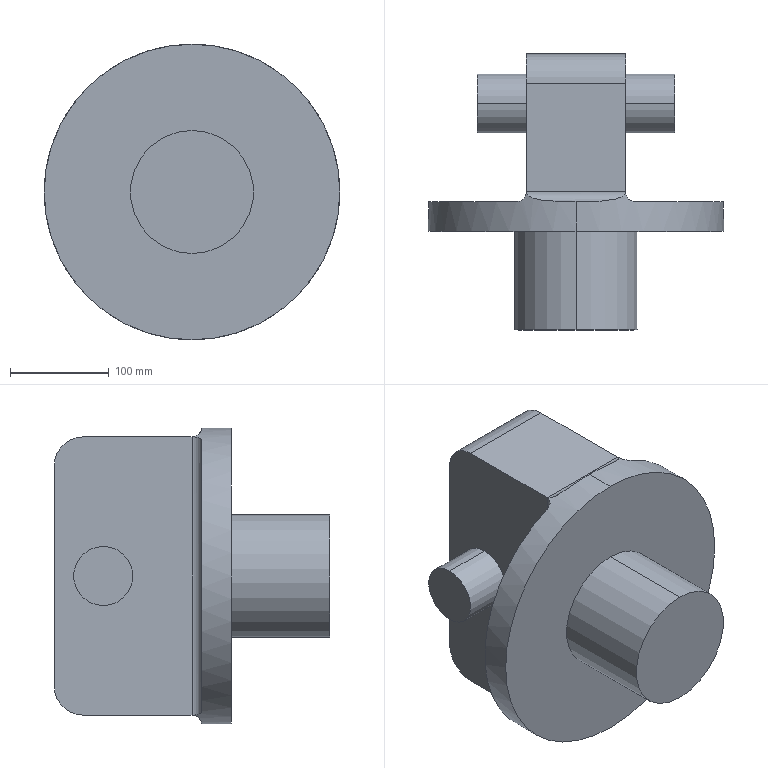Part | SolidWorks | features Revolution 3, ICE 2, BaseBody 1, Fillet 1 | 4 solids | 28 faces | box 300 x 280 x 300 mm | volume 7882331 mm3 | cylinder 14 | plane 14 | commonest cylinder face diameters 60 x6 20 x4 125 x2 300 x2
STEP:
#1=CARTESIAN_POINT('',(0.,100.,-62.5));
#2=VERTEX_POINT('',#1);
#3=CARTESIAN_POINT('',(0.,100.,62.5));
#4=VERTEX_POINT('',#3);
#5=CARTESIAN_POINT('',(0.,100.,0.));
#6=DIRECTION('',(0.,-1.,0.));
#7=DIRECTION('',(0.,0.,-1.));
#8=AXIS2_PLACEMENT_3D('',#5,#6,#7);
#9=CIRCLE('',#8,62.5);
#10=EDGE_CURVE('',#2,#4,#9,.T.);
#11=ORIENTED_EDGE('',*,*,#10,.T.);
#12=CARTESIAN_POINT('',(0.,0.,62.5));
#13=VERTEX_POINT('',#12);
#14=CARTESIAN_POINT('',(0.,100.,62.5));
#15=DIRECTION('',(0.,-1.,0.));
#16=VECTOR('',#15,1000.);
#17=LINE('',#14,#16);
#18=EDGE_CURVE('',#4,#13,#17,.T.);
#19=ORIENTED_EDGE('',*,*,#18,.T.);
#20=CARTESIAN_POINT('',(0.,0.,-62.5));
#21=VERTEX_POINT('',#20);
#22=CARTESIAN_POINT('',(0.,0.,0.));
#23=DIRECTION('',(0.,-1.,0.));
#24=DIRECTION('',(0.,0.,-1.));
#25=AXIS2_PLACEMENT_3D('',#22,#23,#24);
#26=CIRCLE('',#25,62.5);
#27=EDGE_CURVE('',#21,#13,#26,.T.);
#28=ORIENTED_EDGE('',*,*,#27,.F.);
#29=CARTESIAN_POINT('',(0.,100.,-62.5));
#30=DIRECTION('',(0.,-1.,0.));
#31=VECTOR('',#30,1000.);
#32=LINE('',#29,#31);
#33=EDGE_CURVE('',#2,#21,#32,.T.);
#34=ORIENTED_EDGE('',*,*,#33,.F.);
#35=EDGE_LOOP('',(#11,#19,#28,#34));
#36=FACE_OUTER_BOUND('',#35,.T.);
#37=CARTESIAN_POINT('',(0.,100.,0.));
#38=DIRECTION('',(0.,-1.,0.));
#39=DIRECTION('',(0.,0.,-1.));
#40=AXIS2_PLACEMENT_3D('',#37,#38,#39);
#41=CYLINDRICAL_SURFACE('',#40,62.5);
#42=ADVANCED_FACE('',(#36),#41,.T.);
#43=ORIENTED_EDGE('',*,*,#18,.F.);
#44=CARTESIAN_POINT('',(0.,100.,0.));
#45=DIRECTION('',(0.,-1.,0.));
#46=DIRECTION('',(0.,0.,-1.));
#47=AXIS2_PLACEMENT_3D('',#44,#45,#46);
#48=CIRCLE('',#47,62.5);
#49=EDGE_CURVE('',#4,#2,#48,.T.);
#50=ORIENTED_EDGE('',*,*,#49,.T.);
#51=ORIENTED_EDGE('',*,*,#33,.T.);
#52=CARTESIAN_POINT('',(0.,0.,0.));
#53=DIRECTION('',(0.,-1.,0.));
#54=DIRECTION('',(0.,0.,-1.));
#55=AXIS2_PLACEMENT_3D('',#52,#53,#54);
#56=CIRCLE('',#55,62.5);
#57=EDGE_CURVE('',#13,#21,#56,.T.);
#58=ORIENTED_EDGE('',*,*,#57,.F.);
#59=EDGE_LOOP('',(#43,#50,#51,#58));
#60=FACE_OUTER_BOUND('',#59,.T.);
#61=CARTESIAN_POINT('',(0.,100.,0.));
#62=DIRECTION('',(0.,-1.,0.));
#63=DIRECTION('',(0.,0.,-1.));
#64=AXIS2_PLACEMENT_3D('',#61,#62,#63);
#65=CYLINDRICAL_SURFACE('',#64,62.5);
#66=ADVANCED_FACE('',(#60),#65,.T.);
#67=ORIENTED_EDGE('',*,*,#10,.F.);
#68=ORIENTED_EDGE('',*,*,#49,.F.);
#69=EDGE_LOOP('',(#67,#68));
#70=FACE_OUTER_BOUND('',#69,.T.);
#71=CARTESIAN_POINT('',(62.5,100.,0.));
#72=DIRECTION('',(0.,1.,0.));
#73=DIRECTION('',(0.,0.,1.));
#74=AXIS2_PLACEMENT_3D('',#71,#72,#73);
#75=PLANE('',#74);
#76=ADVANCED_FACE('',(#70),#75,.T.);
#77=ORIENTED_EDGE('',*,*,#27,.T.);
#78=ORIENTED_EDGE('',*,*,#57,.T.);
#79=EDGE_LOOP('',(#77,#78));
#80=FACE_OUTER_BOUND('',#79,.T.);
#81=CARTESIAN_POINT('',(0.,0.,0.));
#82=DIRECTION('',(0.,-1.,0.));
#83=DIRECTION('',(0.,0.,-1.));
#84=AXIS2_PLACEMENT_3D('',#81,#82,#83);
#85=PLANE('',#84);
#86=ADVANCED_FACE('',(#80),#85,.T.);
#87=CLOSED_SHELL('',(#42,#66,#76,#86));
#88=MANIFOLD_SOLID_BREP('',#87);
#89=CARTESIAN_POINT('',(50.437,140.,141.266));
#90=VERTEX_POINT('',#89);
#91=CARTESIAN_POINT('',(0.,130.08,150.));
#92=VERTEX_POINT('',#91);
#93=CARTESIAN_POINT('',(50.437,140.,141.266));
#94=CARTESIAN_POINT('',(50.437,139.707,141.266));
#95=CARTESIAN_POINT('',(50.402,139.421,141.279));
#96=CARTESIAN_POINT('',(50.266,138.862,141.327));
#97=CARTESIAN_POINT('',(50.165,138.586,141.363));
#98=CARTESIAN_POINT('',(49.919,138.072,141.45));
#99=CARTESIAN_POINT('',(49.773,137.828,141.502));
#100=CARTESIAN_POINT('',(49.445,137.364,141.617));
#101=CARTESIAN_POINT('',(49.263,137.144,141.68));
#102=CARTESIAN_POINT('',(48.691,136.528,141.878));
#103=CARTESIAN_POINT('',(48.267,136.166,142.023));
#104=CARTESIAN_POINT('',(47.592,135.671,142.25));
#105=CARTESIAN_POINT('',(47.361,135.514,142.327));
#106=CARTESIAN_POINT('',(46.893,135.218,142.482));
#107=CARTESIAN_POINT('',(46.655,135.077,142.56));
#108=CARTESIAN_POINT('',(45.453,134.41,142.951));
#109=CARTESIAN_POINT('',(44.446,133.978,143.268));
#110=CARTESIAN_POINT('',(42.38,133.227,143.893));
#111=CARTESIAN_POINT('',(41.315,132.91,144.202));
#112=CARTESIAN_POINT('',(39.177,132.363,144.798));
#113=CARTESIAN_POINT('',(38.101,132.132,145.085));
#114=CARTESIAN_POINT('',(35.936,131.728,145.636));
#115=CARTESIAN_POINT('',(34.848,131.556,145.9));
#116=CARTESIAN_POINT('',(31.566,131.105,146.658));
#117=CARTESIAN_POINT('',(29.357,130.891,147.117));
#118=CARTESIAN_POINT('',(24.906,130.561,147.935));
#119=CARTESIAN_POINT('',(22.663,130.446,148.296));
#120=CARTESIAN_POINT('',(18.151,130.275,148.915));
#121=CARTESIAN_POINT('',(15.891,130.219,149.173));
#122=CARTESIAN_POINT('',(11.364,130.14,149.586));
#123=CARTESIAN_POINT('',(9.096,130.116,149.741));
#124=CARTESIAN_POINT('',(4.554,130.087,149.948));
#125=CARTESIAN_POINT('',(2.279,130.08,150.));
#126=CARTESIAN_POINT('',(0.,130.08,150.));
#127=B_SPLINE_CURVE_WITH_KNOTS('',3,(#93,#94,#95,#96,#97,#98,#99,#100,#101,#102,#103,#104,#105,#106,#107,#108,#109,#110,#111,#112,#113,#114,#115,#116,#117,#118,#119,#120,#121,#122,#123,#124,#125,#126),.UNSPECIFIED.,.F.,.F.,(4,2,2,2,2,2,2,2,2,2,2,2,2,2,2,2,4),(-0.05456,-0.05371,-0.05285,-0.052,-0.05115,-0.04944,-0.04859,-0.04774,-0.04433,-0.04092,-0.03751,-0.0341,-0.02728,-0.02046,-0.01364,-0.00682,0.),.UNSPECIFIED.);
#128=EDGE_CURVE('',#90,#92,#127,.T.);
#129=ORIENTED_EDGE('',*,*,#128,.T.);
#130=CARTESIAN_POINT('',(0.,100.,150.));
#131=VERTEX_POINT('',#130);
#132=CARTESIAN_POINT('',(0.,130.,150.));
#133=DIRECTION('',(0.,-1.,0.));
#134=VECTOR('',#133,1000.);
#135=LINE('',#132,#134);
#136=EDGE_CURVE('',#92,#131,#135,.T.);
#137=ORIENTED_EDGE('',*,*,#136,.T.);
#138=CARTESIAN_POINT('',(0.,100.,-150.));
#139=VERTEX_POINT('',#138);
#140=CARTESIAN_POINT('',(0.,100.,0.));
#141=DIRECTION('',(0.,-1.,0.));
#142=DIRECTION('',(0.,0.,-1.));
#143=AXIS2_PLACEMENT_3D('',#140,#141,#142);
#144=CIRCLE('',#143,150.);
#145=EDGE_CURVE('',#139,#131,#144,.T.);
#146=ORIENTED_EDGE('',*,*,#145,.F.);
#147=CARTESIAN_POINT('',(0.,130.08,-150.));
#148=VERTEX_POINT('',#147);
#149=CARTESIAN_POINT('',(0.,130.,-150.));
#150=DIRECTION('',(0.,-1.,0.));
#151=VECTOR('',#150,1000.);
#152=LINE('',#149,#151);
#153=EDGE_CURVE('',#148,#139,#152,.T.);
#154=ORIENTED_EDGE('',*,*,#153,.F.);
#155=CARTESIAN_POINT('',(50.437,140.,-141.266));
#156=VERTEX_POINT('',#155);
#157=CARTESIAN_POINT('',(0.,130.08,-150.));
#158=CARTESIAN_POINT('',(2.28,130.08,-150.));
#159=CARTESIAN_POINT('',(4.556,130.087,-149.948));
#160=CARTESIAN_POINT('',(9.102,130.116,-149.741));
#161=CARTESIAN_POINT('',(11.371,130.14,-149.586));
#162=CARTESIAN_POINT('',(15.903,130.219,-149.172));
#163=CARTESIAN_POINT('',(18.165,130.275,-148.913));
#164=CARTESIAN_POINT('',(22.68,130.447,-148.293));
#165=CARTESIAN_POINT('',(24.927,130.562,-147.932));
#166=CARTESIAN_POINT('',(29.397,130.894,-147.109));
#167=CARTESIAN_POINT('',(31.622,131.111,-146.646));
#168=CARTESIAN_POINT('',(34.922,131.567,-145.883));
#169=CARTESIAN_POINT('',(36.016,131.742,-145.616));
#170=CARTESIAN_POINT('',(38.191,132.15,-145.061));
#171=CARTESIAN_POINT('',(39.268,132.384,-144.773));
#172=CARTESIAN_POINT('',(41.395,132.933,-144.179));
#173=CARTESIAN_POINT('',(42.445,133.248,-143.874));
#174=CARTESIAN_POINT('',(43.992,133.814,-143.405));
#175=CARTESIAN_POINT('',(44.502,134.018,-143.248));
#176=CARTESIAN_POINT('',(45.501,134.465,-142.933));
#177=CARTESIAN_POINT('',(45.992,134.707,-142.776));
#178=CARTESIAN_POINT('',(46.947,135.242,-142.465));
#179=CARTESIAN_POINT('',(47.415,135.537,-142.31));
#180=CARTESIAN_POINT('',(48.301,136.194,-142.011));
#181=CARTESIAN_POINT('',(48.719,136.554,-141.868));
#182=CARTESIAN_POINT('',(49.475,137.377,-141.606));
#183=CARTESIAN_POINT('',(49.805,137.83,-141.49));
#184=CARTESIAN_POINT('',(50.171,138.602,-141.361));
#185=CARTESIAN_POINT('',(50.268,138.869,-141.326));
#186=CARTESIAN_POINT('',(50.401,139.422,-141.279));
#187=CARTESIAN_POINT('',(50.437,139.711,-141.266));
#188=CARTESIAN_POINT('',(50.437,140.,-141.266));
#189=B_SPLINE_CURVE_WITH_KNOTS('',3,(#157,#158,#159,#160,#161,#162,#163,#164,#165,#166,#167,#168,#169,#170,#171,#172,#173,#174,#175,#176,#177,#178,#179,#180,#181,#182,#183,#184,#185,#186,#187,#188),.UNSPECIFIED.,.F.,.F.,(4,2,2,2,2,2,2,2,2,2,2,2,2,2,2,4),(0.,0.006824,0.01365,0.02047,0.0273,0.03412,0.03753,0.04094,0.04436,0.04606,0.04777,0.04947,0.05118,0.05289,0.05374,0.05459),.UNSPECIFIED.);
#190=EDGE_CURVE('',#148,#156,#189,.T.);
#191=ORIENTED_EDGE('',*,*,#190,.T.);
#192=CARTESIAN_POINT('',(60.437,130.,-137.286));
#193=VERTEX_POINT('',#192);
#194=CARTESIAN_POINT('',(50.437,140.,-141.266));
#195=CARTESIAN_POINT('',(50.437,139.313,-141.266));
#196=CARTESIAN_POINT('',(50.507,138.639,-141.241));
#197=CARTESIAN_POINT('',(50.713,137.646,-141.167));
#198=CARTESIAN_POINT('',(50.798,137.319,-141.137));
#199=CARTESIAN_POINT('',(51.002,136.669,-141.063));
#200=CARTESIAN_POINT('',(51.121,136.35,-141.02));
#201=CARTESIAN_POINT('',(51.52,135.424,-140.875));
#202=CARTESIAN_POINT('',(51.845,134.841,-140.756));
#203=CARTESIAN_POINT('',(52.417,134.018,-140.544));
#204=CARTESIAN_POINT('',(52.622,133.753,-140.467));
#205=CARTESIAN_POINT('',(53.051,133.251,-140.305));
#206=CARTESIAN_POINT('',(53.277,133.012,-140.22));
#207=CARTESIAN_POINT('',(53.748,132.56,-140.04));
#208=CARTESIAN_POINT('',(53.994,132.346,-139.945));
#209=CARTESIAN_POINT('',(54.506,131.943,-139.747));
#210=CARTESIAN_POINT('',(54.773,131.752,-139.642));
#211=CARTESIAN_POINT('',(55.591,131.229,-139.32));
#212=CARTESIAN_POINT('',(56.159,130.939,-139.092));
#213=CARTESIAN_POINT('',(57.339,130.471,-138.61));
#214=CARTESIAN_POINT('',(57.955,130.293,-138.353));
#215=CARTESIAN_POINT('',(59.188,130.059,-137.83));
#216=CARTESIAN_POINT('',(59.81,130.,-137.562));
#217=CARTESIAN_POINT('',(60.437,130.,-137.286));
#218=B_SPLINE_CURVE_WITH_KNOTS('',3,(#194,#195,#196,#197,#198,#199,#200,#201,#202,#203,#204,#205,#206,#207,#208,#209,#210,#211,#212,#213,#214,#215,#216,#217),.UNSPECIFIED.,.F.,.F.,(4,2,2,2,2,2,2,2,2,2,2,4),(0.,0.002031,0.003046,0.004061,0.006092,0.007107,0.008122,0.009137,0.01015,0.01218,0.01421,0.01624),.UNSPECIFIED.);
#219=EDGE_CURVE('',#156,#193,#218,.T.);
#220=ORIENTED_EDGE('',*,*,#219,.T.);
#221=CARTESIAN_POINT('',(60.437,130.,137.286));
#222=VERTEX_POINT('',#221);
#223=CARTESIAN_POINT('',(0.,130.,0.));
#224=DIRECTION('',(0.,-1.,0.));
#225=DIRECTION('',(0.,0.,-1.));
#226=AXIS2_PLACEMENT_3D('',#223,#224,#225);
#227=CIRCLE('',#226,150.);
#228=EDGE_CURVE('',#193,#222,#227,.T.);
#229=ORIENTED_EDGE('',*,*,#228,.T.);
#230=CARTESIAN_POINT('',(60.437,130.,137.286));
#231=CARTESIAN_POINT('',(59.809,130.,137.562));
#232=CARTESIAN_POINT('',(59.189,130.059,137.83));
#233=CARTESIAN_POINT('',(58.268,130.233,138.221));
#234=CARTESIAN_POINT('',(57.963,130.306,138.349));
#235=CARTESIAN_POINT('',(57.356,130.481,138.602));
#236=CARTESIAN_POINT('',(57.053,130.585,138.726));
#237=CARTESIAN_POINT('',(56.161,130.938,139.091));
#238=CARTESIAN_POINT('',(55.593,131.228,139.319));
#239=CARTESIAN_POINT('',(54.782,131.746,139.639));
#240=CARTESIAN_POINT('',(54.519,131.933,139.742));
#241=CARTESIAN_POINT('',(54.007,132.335,139.94));
#242=CARTESIAN_POINT('',(53.757,132.552,140.037));
#243=CARTESIAN_POINT('',(53.044,133.235,140.309));
#244=CARTESIAN_POINT('',(52.616,133.734,140.47));
#245=CARTESIAN_POINT('',(52.047,134.549,140.681));
#246=CARTESIAN_POINT('',(51.87,134.832,140.746));
#247=CARTESIAN_POINT('',(51.541,135.42,140.867));
#248=CARTESIAN_POINT('',(51.391,135.725,140.922));
#249=CARTESIAN_POINT('',(50.991,136.651,141.067));
#250=CARTESIAN_POINT('',(50.787,137.293,141.141));
#251=CARTESIAN_POINT('',(50.579,138.291,141.215));
#252=CARTESIAN_POINT('',(50.526,138.632,141.234));
#253=CARTESIAN_POINT('',(50.455,139.314,141.26));
#254=CARTESIAN_POINT('',(50.437,139.656,141.266));
#255=CARTESIAN_POINT('',(50.437,140.,141.266));
#256=B_SPLINE_CURVE_WITH_KNOTS('',3,(#230,#231,#232,#233,#234,#235,#236,#237,#238,#239,#240,#241,#242,#243,#244,#245,#246,#247,#248,#249,#250,#251,#252,#253,#254,#255),.UNSPECIFIED.,.F.,.F.,(4,2,2,2,2,2,2,2,2,2,2,2,4),(0.,0.00203,0.003046,0.004061,0.006091,0.007107,0.008122,0.01015,0.01117,0.01218,0.01421,0.01523,0.01624),.UNSPECIFIED.);
#257=EDGE_CURVE('',#222,#90,#256,.T.);
#258=ORIENTED_EDGE('',*,*,#257,.T.);
#259=EDGE_LOOP('',(#129,#137,#146,#154,#191,#220,#229,#258));
#260=FACE_OUTER_BOUND('',#259,.T.);
#261=CARTESIAN_POINT('',(0.,130.,0.));
#262=DIRECTION('',(0.,-1.,0.));
#263=DIRECTION('',(0.,0.,-1.));
#264=AXIS2_PLACEMENT_3D('',#261,#262,#263);
#265=CYLINDRICAL_SURFACE('',#264,150.);
#266=ADVANCED_FACE('',(#260),#265,.T.);
#267=ORIENTED_EDGE('',*,*,#136,.F.);
#268=CARTESIAN_POINT('',(-50.437,140.,141.266));
#269=VERTEX_POINT('',#268);
#270=CARTESIAN_POINT('',(0.,130.08,150.));
#271=CARTESIAN_POINT('',(-2.28,130.08,150.));
#272=CARTESIAN_POINT('',(-4.556,130.087,149.948));
#273=CARTESIAN_POINT('',(-9.102,130.116,149.741));
#274=CARTESIAN_POINT('',(-11.371,130.14,149.586));
#275=CARTESIAN_POINT('',(-15.903,130.219,149.172));
#276=CARTESIAN_POINT('',(-18.165,130.275,148.913));
#277=CARTESIAN_POINT('',(-22.68,130.447,148.293));
#278=CARTESIAN_POINT('',(-24.927,130.562,147.932));
#279=CARTESIAN_POINT('',(-29.397,130.894,147.109));
#280=CARTESIAN_POINT('',(-31.622,131.111,146.646));
#281=CARTESIAN_POINT('',(-34.922,131.567,145.883));
#282=CARTESIAN_POINT('',(-36.016,131.742,145.616));
#283=CARTESIAN_POINT('',(-38.191,132.15,145.061));
#284=CARTESIAN_POINT('',(-39.268,132.384,144.773));
#285=CARTESIAN_POINT('',(-41.395,132.933,144.179));
#286=CARTESIAN_POINT('',(-42.445,133.248,143.874));
#287=CARTESIAN_POINT('',(-43.992,133.814,143.405));
#288=CARTESIAN_POINT('',(-44.502,134.018,143.248));
#289=CARTESIAN_POINT('',(-45.501,134.465,142.933));
#290=CARTESIAN_POINT('',(-45.992,134.707,142.776));
#291=CARTESIAN_POINT('',(-46.947,135.242,142.465));
#292=CARTESIAN_POINT('',(-47.415,135.537,142.31));
#293=CARTESIAN_POINT('',(-48.301,136.194,142.011));
#294=CARTESIAN_POINT('',(-48.719,136.554,141.868));
#295=CARTESIAN_POINT('',(-49.475,137.377,141.606));
#296=CARTESIAN_POINT('',(-49.805,137.83,141.49));
#297=CARTESIAN_POINT('',(-50.171,138.602,141.361));
#298=CARTESIAN_POINT('',(-50.268,138.869,141.326));
#299=CARTESIAN_POINT('',(-50.401,139.422,141.279));
#300=CARTESIAN_POINT('',(-50.437,139.711,141.266));
#301=CARTESIAN_POINT('',(-50.437,140.,141.266));
#302=B_SPLINE_CURVE_WITH_KNOTS('',3,(#270,#271,#272,#273,#274,#275,#276,#277,#278,#279,#280,#281,#282,#283,#284,#285,#286,#287,#288,#289,#290,#291,#292,#293,#294,#295,#296,#297,#298,#299,#300,#301),.UNSPECIFIED.,.F.,.F.,(4,2,2,2,2,2,2,2,2,2,2,2,2,2,2,4),(0.,0.006824,0.01365,0.02047,0.0273,0.03412,0.03753,0.04094,0.04436,0.04606,0.04777,0.04947,0.05118,0.05289,0.05374,0.05459),.UNSPECIFIED.);
#303=EDGE_CURVE('',#92,#269,#302,.T.);
#304=ORIENTED_EDGE('',*,*,#303,.T.);
#305=CARTESIAN_POINT('',(-60.437,130.,137.286));
#306=VERTEX_POINT('',#305);
#307=CARTESIAN_POINT('',(-50.437,140.,141.266));
#308=CARTESIAN_POINT('',(-50.437,139.313,141.266));
#309=CARTESIAN_POINT('',(-50.507,138.639,141.241));
#310=CARTESIAN_POINT('',(-50.713,137.646,141.167));
#311=CARTESIAN_POINT('',(-50.798,137.319,141.137));
#312=CARTESIAN_POINT('',(-51.002,136.669,141.063));
#313=CARTESIAN_POINT('',(-51.121,136.35,141.02));
#314=CARTESIAN_POINT('',(-51.52,135.424,140.875));
#315=CARTESIAN_POINT('',(-51.845,134.841,140.756));
#316=CARTESIAN_POINT('',(-52.417,134.018,140.544));
#317=CARTESIAN_POINT('',(-52.622,133.753,140.467));
#318=CARTESIAN_POINT('',(-53.051,133.251,140.305));
#319=CARTESIAN_POINT('',(-53.277,133.012,140.22));
#320=CARTESIAN_POINT('',(-53.748,132.56,140.04));
#321=CARTESIAN_POINT('',(-53.994,132.346,139.945));
#322=CARTESIAN_POINT('',(-54.506,131.943,139.747));
#323=CARTESIAN_POINT('',(-54.773,131.752,139.642));
#324=CARTESIAN_POINT('',(-55.591,131.229,139.32));
#325=CARTESIAN_POINT('',(-56.159,130.939,139.092));
#326=CARTESIAN_POINT('',(-57.339,130.471,138.61));
#327=CARTESIAN_POINT('',(-57.955,130.293,138.353));
#328=CARTESIAN_POINT('',(-59.188,130.059,137.83));
#329=CARTESIAN_POINT('',(-59.81,130.,137.562));
#330=CARTESIAN_POINT('',(-60.437,130.,137.286));
#331=B_SPLINE_CURVE_WITH_KNOTS('',3,(#307,#308,#309,#310,#311,#312,#313,#314,#315,#316,#317,#318,#319,#320,#321,#322,#323,#324,#325,#326,#327,#328,#329,#330),.UNSPECIFIED.,.F.,.F.,(4,2,2,2,2,2,2,2,2,2,2,4),(0.,0.002031,0.003046,0.004061,0.006092,0.007107,0.008122,0.009137,0.01015,0.01218,0.01421,0.01624),.UNSPECIFIED.);
#332=EDGE_CURVE('',#269,#306,#331,.T.);
#333=ORIENTED_EDGE('',*,*,#332,.T.);
#334=CARTESIAN_POINT('',(-60.437,130.,-137.286));
#335=VERTEX_POINT('',#334);
#336=CARTESIAN_POINT('',(0.,130.,0.));
#337=DIRECTION('',(0.,-1.,0.));
#338=DIRECTION('',(0.,0.,-1.));
#339=AXIS2_PLACEMENT_3D('',#336,#337,#338);
#340=CIRCLE('',#339,150.);
#341=EDGE_CURVE('',#306,#335,#340,.T.);
#342=ORIENTED_EDGE('',*,*,#341,.T.);
#343=CARTESIAN_POINT('',(-50.437,140.,-141.266));
#344=VERTEX_POINT('',#343);
#345=CARTESIAN_POINT('',(-60.437,130.,-137.286));
#346=CARTESIAN_POINT('',(-59.809,130.,-137.562));
#347=CARTESIAN_POINT('',(-59.189,130.059,-137.83));
#348=CARTESIAN_POINT('',(-58.268,130.233,-138.221));
#349=CARTESIAN_POINT('',(-57.963,130.306,-138.349));
#350=CARTESIAN_POINT('',(-57.356,130.481,-138.602));
#351=CARTESIAN_POINT('',(-57.053,130.585,-138.726));
#352=CARTESIAN_POINT('',(-56.161,130.938,-139.091));
#353=CARTESIAN_POINT('',(-55.593,131.228,-139.319));
#354=CARTESIAN_POINT('',(-54.782,131.746,-139.639));
#355=CARTESIAN_POINT('',(-54.519,131.933,-139.742));
#356=CARTESIAN_POINT('',(-54.007,132.335,-139.94));
#357=CARTESIAN_POINT('',(-53.757,132.552,-140.037));
#358=CARTESIAN_POINT('',(-53.044,133.235,-140.309));
#359=CARTESIAN_POINT('',(-52.616,133.734,-140.47));
#360=CARTESIAN_POINT('',(-52.047,134.549,-140.681));
#361=CARTESIAN_POINT('',(-51.87,134.832,-140.746));
#362=CARTESIAN_POINT('',(-51.541,135.42,-140.867));
#363=CARTESIAN_POINT('',(-51.391,135.725,-140.922));
#364=CARTESIAN_POINT('',(-50.991,136.651,-141.067));
#365=CARTESIAN_POINT('',(-50.787,137.293,-141.141));
#366=CARTESIAN_POINT('',(-50.579,138.291,-141.215));
#367=CARTESIAN_POINT('',(-50.526,138.632,-141.234));
#368=CARTESIAN_POINT('',(-50.455,139.314,-141.26));
#369=CARTESIAN_POINT('',(-50.437,139.656,-141.266));
#370=CARTESIAN_POINT('',(-50.437,140.,-141.266));
#371=B_SPLINE_CURVE_WITH_KNOTS('',3,(#345,#346,#347,#348,#349,#350,#351,#352,#353,#354,#355,#356,#357,#358,#359,#360,#361,#362,#363,#364,#365,#366,#367,#368,#369,#370),.UNSPECIFIED.,.F.,.F.,(4,2,2,2,2,2,2,2,2,2,2,2,4),(0.,0.00203,0.003046,0.004061,0.006091,0.007107,0.008122,0.01015,0.01117,0.01218,0.01421,0.01523,0.01624),.UNSPECIFIED.);
#372=EDGE_CURVE('',#335,#344,#371,.T.);
#373=ORIENTED_EDGE('',*,*,#372,.T.);
#374=CARTESIAN_POINT('',(-50.437,140.,-141.266));
#375=CARTESIAN_POINT('',(-50.437,139.707,-141.266));
#376=CARTESIAN_POINT('',(-50.402,139.421,-141.279));
#377=CARTESIAN_POINT('',(-50.266,138.862,-141.327));
#378=CARTESIAN_POINT('',(-50.165,138.586,-141.363));
#379=CARTESIAN_POINT('',(-49.919,138.072,-141.45));
#380=CARTESIAN_POINT('',(-49.773,137.828,-141.502));
#381=CARTESIAN_POINT('',(-49.445,137.364,-141.617));
#382=CARTESIAN_POINT('',(-49.263,137.144,-141.68));
#383=CARTESIAN_POINT('',(-48.691,136.528,-141.878));
#384=CARTESIAN_POINT('',(-48.267,136.166,-142.023));
#385=CARTESIAN_POINT('',(-47.592,135.671,-142.25));
#386=CARTESIAN_POINT('',(-47.361,135.514,-142.327));
#387=CARTESIAN_POINT('',(-46.893,135.218,-142.482));
#388=CARTESIAN_POINT('',(-46.655,135.077,-142.56));
#389=CARTESIAN_POINT('',(-45.453,134.41,-142.951));
#390=CARTESIAN_POINT('',(-44.446,133.978,-143.268));
#391=CARTESIAN_POINT('',(-42.38,133.227,-143.893));
#392=CARTESIAN_POINT('',(-41.315,132.91,-144.202));
#393=CARTESIAN_POINT('',(-39.177,132.363,-144.798));
#394=CARTESIAN_POINT('',(-38.101,132.132,-145.085));
#395=CARTESIAN_POINT('',(-35.936,131.728,-145.636));
#396=CARTESIAN_POINT('',(-34.848,131.556,-145.9));
#397=CARTESIAN_POINT('',(-31.566,131.105,-146.658));
#398=CARTESIAN_POINT('',(-29.357,130.891,-147.117));
#399=CARTESIAN_POINT('',(-24.906,130.561,-147.935));
#400=CARTESIAN_POINT('',(-22.663,130.446,-148.296));
#401=CARTESIAN_POINT('',(-18.151,130.275,-148.915));
#402=CARTESIAN_POINT('',(-15.891,130.219,-149.173));
#403=CARTESIAN_POINT('',(-11.364,130.14,-149.586));
#404=CARTESIAN_POINT('',(-9.096,130.116,-149.741));
#405=CARTESIAN_POINT('',(-4.554,130.087,-149.948));
#406=CARTESIAN_POINT('',(-2.279,130.08,-150.));
#407=CARTESIAN_POINT('',(0.,130.08,-150.));
#408=B_SPLINE_CURVE_WITH_KNOTS('',3,(#374,#375,#376,#377,#378,#379,#380,#381,#382,#383,#384,#385,#386,#387,#388,#389,#390,#391,#392,#393,#394,#395,#396,#397,#398,#399,#400,#401,#402,#403,#404,#405,#406,#407),.UNSPECIFIED.,.F.,.F.,(4,2,2,2,2,2,2,2,2,2,2,2,2,2,2,2,4),(-0.05456,-0.05371,-0.05285,-0.052,-0.05115,-0.04944,-0.04859,-0.04774,-0.04433,-0.04092,-0.03751,-0.0341,-0.02728,-0.02046,-0.01364,-0.00682,0.),.UNSPECIFIED.);
#409=EDGE_CURVE('',#344,#148,#408,.T.);
#410=ORIENTED_EDGE('',*,*,#409,.T.);
#411=ORIENTED_EDGE('',*,*,#153,.T.);
#412=CARTESIAN_POINT('',(0.,100.,0.));
#413=DIRECTION('',(0.,-1.,0.));
#414=DIRECTION('',(0.,0.,-1.));
#415=AXIS2_PLACEMENT_3D('',#412,#413,#414);
#416=CIRCLE('',#415,150.);
#417=EDGE_CURVE('',#131,#139,#416,.T.);
#418=ORIENTED_EDGE('',*,*,#417,.F.);
#419=EDGE_LOOP('',(#267,#304,#333,#342,#373,#410,#411,#418));
#420=FACE_OUTER_BOUND('',#419,.T.);
#421=CARTESIAN_POINT('',(0.,130.,0.));
#422=DIRECTION('',(0.,-1.,0.));
#423=DIRECTION('',(0.,0.,-1.));
#424=AXIS2_PLACEMENT_3D('',#421,#422,#423);
#425=CYLINDRICAL_SURFACE('',#424,150.);
#426=ADVANCED_FACE('',(#420),#425,.T.);
#427=CARTESIAN_POINT('',(50.437,140.,-141.266));
#428=DIRECTION('',(-1.,0.,0.));
#429=VECTOR('',#428,1000.);
#430=LINE('',#427,#429);
#431=EDGE_CURVE('',#156,#344,#430,.T.);
#432=ORIENTED_EDGE('',*,*,#431,.F.);
#433=ORIENTED_EDGE('',*,*,#190,.F.);
#434=ORIENTED_EDGE('',*,*,#409,.F.);
#435=EDGE_LOOP('',(#432,#433,#434));
#436=FACE_OUTER_BOUND('',#435,.T.);
#437=CARTESIAN_POINT('',(50.437,140.,-151.266));
#438=DIRECTION('',(-1.,0.,0.));
#439=DIRECTION('',(0.,0.,1.));
#440=AXIS2_PLACEMENT_3D('',#437,#438,#439);
#441=CYLINDRICAL_SURFACE('',#440,10.);
#442=ADVANCED_FACE('',(#436),#441,.F.);
#443=CARTESIAN_POINT('',(50.437,140.,141.266));
#444=DIRECTION('',(1.,0.,0.));
#445=VECTOR('',#444,1000.);
#446=LINE('',#443,#445);
#447=EDGE_CURVE('',#269,#90,#446,.T.);
#448=ORIENTED_EDGE('',*,*,#447,.F.);
#449=ORIENTED_EDGE('',*,*,#303,.F.);
#450=ORIENTED_EDGE('',*,*,#128,.F.);
#451=EDGE_LOOP('',(#448,#449,#450));
#452=FACE_OUTER_BOUND('',#451,.T.);
#453=CARTESIAN_POINT('',(50.437,140.,151.266));
#454=DIRECTION('',(1.,0.,0.));
#455=DIRECTION('',(0.,0.,-1.));
#456=AXIS2_PLACEMENT_3D('',#453,#454,#455);
#457=CYLINDRICAL_SURFACE('',#456,10.);
#458=ADVANCED_FACE('',(#452),#457,.F.);
#459=ORIENTED_EDGE('',*,*,#372,.F.);
#460=CARTESIAN_POINT('',(-60.437,130.,0.));
#461=DIRECTION('',(0.,0.,-1.));
#462=VECTOR('',#461,1000.);
#463=LINE('',#460,#462);
#464=EDGE_CURVE('',#306,#335,#463,.T.);
#465=ORIENTED_EDGE('',*,*,#464,.F.);
#466=ORIENTED_EDGE('',*,*,#332,.F.);
#467=CARTESIAN_POINT('',(-50.437,140.,-141.266));
#468=DIRECTION('',(0.,0.,1.));
#469=VECTOR('',#468,1000.);
#470=LINE('',#467,#469);
#471=EDGE_CURVE('',#344,#269,#470,.T.);
#472=ORIENTED_EDGE('',*,*,#471,.F.);
#473=EDGE_LOOP('',(#459,#465,#466,#472));
#474=FACE_OUTER_BOUND('',#473,.T.);
#475=CARTESIAN_POINT('',(-60.437,140.,-141.266));
#476=DIRECTION('',(0.,0.,1.));
#477=DIRECTION('',(1.,0.,0.));
#478=AXIS2_PLACEMENT_3D('',#475,#476,#477);
#479=CYLINDRICAL_SURFACE('',#478,10.);
#480=ADVANCED_FACE('',(#474),#479,.F.);
#481=ORIENTED_EDGE('',*,*,#257,.F.);
#482=CARTESIAN_POINT('',(60.437,130.,0.));
#483=DIRECTION('',(0.,0.,1.));
#484=VECTOR('',#483,1000.);
#485=LINE('',#482,#484);
#486=EDGE_CURVE('',#193,#222,#485,.T.);
#487=ORIENTED_EDGE('',*,*,#486,.F.);
#488=ORIENTED_EDGE('',*,*,#219,.F.);
#489=CARTESIAN_POINT('',(50.437,140.,-141.266));
#490=DIRECTION('',(0.,0.,-1.));
#491=VECTOR('',#490,1000.);
#492=LINE('',#489,#491);
#493=EDGE_CURVE('',#90,#156,#492,.T.);
#494=ORIENTED_EDGE('',*,*,#493,.F.);
#495=EDGE_LOOP('',(#481,#487,#488,#494));
#496=FACE_OUTER_BOUND('',#495,.T.);
#497=CARTESIAN_POINT('',(60.437,140.,-141.266));
#498=DIRECTION('',(0.,0.,-1.));
#499=DIRECTION('',(-1.,0.,0.));
#500=AXIS2_PLACEMENT_3D('',#497,#498,#499);
#501=CYLINDRICAL_SURFACE('',#500,10.);
#502=ADVANCED_FACE('',(#496),#501,.F.);
#503=ORIENTED_EDGE('',*,*,#341,.F.);
#504=ORIENTED_EDGE('',*,*,#464,.T.);
#505=EDGE_LOOP('',(#503,#504));
#506=FACE_OUTER_BOUND('',#505,.T.);
#507=CARTESIAN_POINT('',(0.,130.,0.));
#508=DIRECTION('',(0.,-1.,0.));
#509=DIRECTION('',(0.,0.,-1.));
#510=AXIS2_PLACEMENT_3D('',#507,#508,#509);
#511=PLANE('',#510);
#512=ADVANCED_FACE('',(#506),#511,.F.);
#513=ORIENTED_EDGE('',*,*,#228,.F.);
#514=ORIENTED_EDGE('',*,*,#486,.T.);
#515=EDGE_LOOP('',(#513,#514));
#516=FACE_OUTER_BOUND('',#515,.T.);
#517=CARTESIAN_POINT('',(0.,130.,0.));
#518=DIRECTION('',(0.,-1.,0.));
#519=DIRECTION('',(0.,0.,-1.));
#520=AXIS2_PLACEMENT_3D('',#517,#518,#519);
#521=PLANE('',#520);
#522=ADVANCED_FACE('',(#516),#521,.F.);
#523=ORIENTED_EDGE('',*,*,#145,.T.);
#524=ORIENTED_EDGE('',*,*,#417,.T.);
#525=EDGE_LOOP('',(#523,#524));
#526=FACE_OUTER_BOUND('',#525,.T.);
#527=CARTESIAN_POINT('',(0.,100.,0.));
#528=DIRECTION('',(0.,-1.,0.));
#529=DIRECTION('',(0.,0.,-1.));
#530=AXIS2_PLACEMENT_3D('',#527,#528,#529);
#531=PLANE('',#530);
#532=ADVANCED_FACE('',(#526),#531,.T.);
#533=CARTESIAN_POINT('',(-50.437,250.,-141.266));
#534=VERTEX_POINT('',#533);
#535=CARTESIAN_POINT('',(-50.437,280.,-141.266));
#536=DIRECTION('',(0.,-1.,0.));
#537=VECTOR('',#536,1000.);
#538=LINE('',#535,#537);
#539=EDGE_CURVE('',#534,#344,#538,.T.);
#540=ORIENTED_EDGE('',*,*,#539,.F.);
#541=CARTESIAN_POINT('',(50.437,250.,-141.266));
#542=VERTEX_POINT('',#541);
#543=CARTESIAN_POINT('',(-50.437,250.,-141.266));
#544=DIRECTION('',(1.,0.,0.));
#545=VECTOR('',#544,1000.);
#546=LINE('',#543,#545);
#547=EDGE_CURVE('',#534,#542,#546,.T.);
#548=ORIENTED_EDGE('',*,*,#547,.T.);
#549=CARTESIAN_POINT('',(50.437,280.,-141.266));
#550=DIRECTION('',(0.,-1.,0.));
#551=VECTOR('',#550,1000.);
#552=LINE('',#549,#551);
#553=EDGE_CURVE('',#542,#156,#552,.T.);
#554=ORIENTED_EDGE('',*,*,#553,.T.);
#555=ORIENTED_EDGE('',*,*,#431,.T.);
#556=EDGE_LOOP('',(#540,#548,#554,#555));
#557=FACE_OUTER_BOUND('',#556,.T.);
#558=CARTESIAN_POINT('',(-50.437,280.,-141.266));
#559=DIRECTION('',(0.,0.,1.));
#560=DIRECTION('',(1.,0.,0.));
#561=AXIS2_PLACEMENT_3D('',#558,#559,#560);
#562=PLANE('',#561);
#563=ADVANCED_FACE('',(#557),#562,.F.);
#564=CARTESIAN_POINT('',(-50.437,250.,141.266));
#565=VERTEX_POINT('',#564);
#566=CARTESIAN_POINT('',(-50.437,280.,141.266));
#567=DIRECTION('',(0.,-1.,0.));
#568=VECTOR('',#567,1000.);
#569=LINE('',#566,#568);
#570=EDGE_CURVE('',#565,#269,#569,.T.);
#571=ORIENTED_EDGE('',*,*,#570,.F.);
#572=CARTESIAN_POINT('',(-50.437,280.,111.266));
#573=VERTEX_POINT('',#572);
#574=CARTESIAN_POINT('',(-50.437,250.,111.266));
#575=DIRECTION('',(-1.,0.,0.));
#576=DIRECTION('',(0.,0.,-1.));
#577=AXIS2_PLACEMENT_3D('',#574,#575,#576);
#578=CIRCLE('',#577,30.);
#579=EDGE_CURVE('',#565,#573,#578,.T.);
#580=ORIENTED_EDGE('',*,*,#579,.T.);
#581=CARTESIAN_POINT('',(-50.437,280.,-111.266));
#582=VERTEX_POINT('',#581);
#583=CARTESIAN_POINT('',(-50.437,280.,141.266));
#584=DIRECTION('',(0.,0.,1.));
#585=VECTOR('',#584,1000.);
#586=LINE('',#583,#585);
#587=EDGE_CURVE('',#582,#573,#586,.T.);
#588=ORIENTED_EDGE('',*,*,#587,.F.);
#589=CARTESIAN_POINT('',(-50.437,250.,-111.266));
#590=DIRECTION('',(-1.,0.,0.));
#591=DIRECTION('',(0.,0.,-1.));
#592=AXIS2_PLACEMENT_3D('',#589,#590,#591);
#593=CIRCLE('',#592,30.);
#594=EDGE_CURVE('',#582,#534,#593,.T.);
#595=ORIENTED_EDGE('',*,*,#594,.T.);
#596=ORIENTED_EDGE('',*,*,#539,.T.);
#597=ORIENTED_EDGE('',*,*,#471,.T.);
#598=EDGE_LOOP('',(#571,#580,#588,#595,#596,#597));
#599=FACE_OUTER_BOUND('',#598,.T.);
#600=CARTESIAN_POINT('',(-50.437,280.,141.266));
#601=DIRECTION('',(1.,0.,0.));
#602=DIRECTION('',(0.,0.,-1.));
#603=AXIS2_PLACEMENT_3D('',#600,#601,#602);
#604=PLANE('',#603);
#605=ADVANCED_FACE('',(#599),#604,.F.);
#606=CARTESIAN_POINT('',(50.437,250.,141.266));
#607=VERTEX_POINT('',#606);
#608=CARTESIAN_POINT('',(50.437,280.,141.266));
#609=DIRECTION('',(0.,-1.,0.));
#610=VECTOR('',#609,1000.);
#611=LINE('',#608,#610);
#612=EDGE_CURVE('',#607,#90,#611,.T.);
#613=ORIENTED_EDGE('',*,*,#612,.F.);
#614=CARTESIAN_POINT('',(50.437,250.,141.266));
#615=DIRECTION('',(-1.,0.,0.));
#616=VECTOR('',#615,1000.);
#617=LINE('',#614,#616);
#618=EDGE_CURVE('',#607,#565,#617,.T.);
#619=ORIENTED_EDGE('',*,*,#618,.T.);
#620=ORIENTED_EDGE('',*,*,#570,.T.);
#621=ORIENTED_EDGE('',*,*,#447,.T.);
#622=EDGE_LOOP('',(#613,#619,#620,#621));
#623=FACE_OUTER_BOUND('',#622,.T.);
#624=CARTESIAN_POINT('',(50.437,280.,141.266));
#625=DIRECTION('',(0.,0.,-1.));
#626=DIRECTION('',(-1.,0.,0.));
#627=AXIS2_PLACEMENT_3D('',#624,#625,#626);
#628=PLANE('',#627);
#629=ADVANCED_FACE('',(#623),#628,.F.);
#630=CARTESIAN_POINT('',(50.437,280.,111.266));
#631=VERTEX_POINT('',#630);
#632=CARTESIAN_POINT('',(50.437,280.,-111.266));
#633=VERTEX_POINT('',#632);
#634=CARTESIAN_POINT('',(50.437,280.,-141.266));
#635=DIRECTION('',(0.,0.,-1.));
#636=VECTOR('',#635,1000.);
#637=LINE('',#634,#636);
#638=EDGE_CURVE('',#631,#633,#637,.T.);
#639=ORIENTED_EDGE('',*,*,#638,.F.);
#640=CARTESIAN_POINT('',(50.437,250.,111.266));
#641=DIRECTION('',(1.,0.,0.));
#642=DIRECTION('',(0.,0.,1.));
#643=AXIS2_PLACEMENT_3D('',#640,#641,#642);
#644=CIRCLE('',#643,30.);
#645=EDGE_CURVE('',#631,#607,#644,.T.);
#646=ORIENTED_EDGE('',*,*,#645,.T.);
#647=ORIENTED_EDGE('',*,*,#612,.T.);
#648=ORIENTED_EDGE('',*,*,#493,.T.);
#649=ORIENTED_EDGE('',*,*,#553,.F.);
#650=CARTESIAN_POINT('',(50.437,250.,-111.266));
#651=DIRECTION('',(1.,0.,0.));
#652=DIRECTION('',(0.,0.,1.));
#653=AXIS2_PLACEMENT_3D('',#650,#651,#652);
#654=CIRCLE('',#653,30.);
#655=EDGE_CURVE('',#542,#633,#654,.T.);
#656=ORIENTED_EDGE('',*,*,#655,.T.);
#657=EDGE_LOOP('',(#639,#646,#647,#648,#649,#656));
#658=FACE_OUTER_BOUND('',#657,.T.);
#659=CARTESIAN_POINT('',(50.437,280.,-141.266));
#660=DIRECTION('',(-1.,0.,0.));
#661=DIRECTION('',(0.,0.,1.));
#662=AXIS2_PLACEMENT_3D('',#659,#660,#661);
#663=PLANE('',#662);
#664=ADVANCED_FACE('',(#658),#663,.F.);
#665=ORIENTED_EDGE('',*,*,#587,.T.);
#666=CARTESIAN_POINT('',(0.,280.,111.266));
#667=DIRECTION('',(1.,0.,0.));
#668=VECTOR('',#667,1000.);
#669=LINE('',#666,#668);
#670=EDGE_CURVE('',#573,#631,#669,.T.);
#671=ORIENTED_EDGE('',*,*,#670,.T.);
#672=ORIENTED_EDGE('',*,*,#638,.T.);
#673=CARTESIAN_POINT('',(0.,280.,-111.266));
#674=DIRECTION('',(-1.,0.,0.));
#675=VECTOR('',#674,1000.);
#676=LINE('',#673,#675);
#677=EDGE_CURVE('',#633,#582,#676,.T.);
#678=ORIENTED_EDGE('',*,*,#677,.T.);
#679=EDGE_LOOP('',(#665,#671,#672,#678));
#680=FACE_OUTER_BOUND('',#679,.T.);
#681=CARTESIAN_POINT('',(0.,280.,0.));
#682=DIRECTION('',(0.,-1.,0.));
#683=DIRECTION('',(0.,0.,-1.));
#684=AXIS2_PLACEMENT_3D('',#681,#682,#683);
#685=PLANE('',#684);
#686=ADVANCED_FACE('',(#680),#685,.F.);
#687=ORIENTED_EDGE('',*,*,#579,.F.);
#688=ORIENTED_EDGE('',*,*,#618,.F.);
#689=ORIENTED_EDGE('',*,*,#645,.F.);
#690=ORIENTED_EDGE('',*,*,#670,.F.);
#691=EDGE_LOOP('',(#687,#688,#689,#690));
#692=FACE_OUTER_BOUND('',#691,.T.);
#693=CARTESIAN_POINT('',(0.,250.,111.266));
#694=DIRECTION('',(1.,0.,0.));
#695=DIRECTION('',(0.,0.,-1.));
#696=AXIS2_PLACEMENT_3D('',#693,#694,#695);
#697=CYLINDRICAL_SURFACE('',#696,30.);
#698=ADVANCED_FACE('',(#692),#697,.T.);
#699=ORIENTED_EDGE('',*,*,#655,.F.);
#700=ORIENTED_EDGE('',*,*,#547,.F.);
#701=ORIENTED_EDGE('',*,*,#594,.F.);
#702=ORIENTED_EDGE('',*,*,#677,.F.);
#703=EDGE_LOOP('',(#699,#700,#701,#702));
#704=FACE_OUTER_BOUND('',#703,.T.);
#705=CARTESIAN_POINT('',(0.,250.,-111.266));
#706=DIRECTION('',(-1.,0.,0.));
#707=DIRECTION('',(0.,0.,1.));
#708=AXIS2_PLACEMENT_3D('',#705,#706,#707);
#709=CYLINDRICAL_SURFACE('',#708,30.);
#710=ADVANCED_FACE('',(#704),#709,.T.);
#711=CLOSED_SHELL('',(#266,#426,#442,#458,#480,#502,#512,#522,#532,#563,#605,#629,#664,#686,#698,#710));
#712=MANIFOLD_SOLID_BREP('',#711);
#713=CARTESIAN_POINT('',(-50.437,230.,30.));
#714=VERTEX_POINT('',#713);
#715=CARTESIAN_POINT('',(-50.437,230.,-30.));
#716=VERTEX_POINT('',#715);
#717=CARTESIAN_POINT('',(-50.437,230.,0.));
#718=DIRECTION('',(-1.,0.,0.));
#719=DIRECTION('',(0.,0.,1.));
#720=AXIS2_PLACEMENT_3D('',#717,#718,#719);
#721=CIRCLE('',#720,30.);
#722=EDGE_CURVE('',#714,#716,#721,.T.);
#723=ORIENTED_EDGE('',*,*,#722,.T.);
#724=CARTESIAN_POINT('',(-100.435,230.,-30.));
#725=VERTEX_POINT('',#724);
#726=CARTESIAN_POINT('',(-50.437,230.,-30.));
#727=DIRECTION('',(-1.,0.,0.));
#728=VECTOR('',#727,1000.);
#729=LINE('',#726,#728);
#730=EDGE_CURVE('',#716,#725,#729,.T.);
#731=ORIENTED_EDGE('',*,*,#730,.T.);
#732=CARTESIAN_POINT('',(-100.435,230.,30.));
#733=VERTEX_POINT('',#732);
#734=CARTESIAN_POINT('',(-100.435,230.,0.));
#735=DIRECTION('',(-1.,0.,0.));
#736=DIRECTION('',(0.,0.,1.));
#737=AXIS2_PLACEMENT_3D('',#734,#735,#736);
#738=CIRCLE('',#737,30.);
#739=EDGE_CURVE('',#733,#725,#738,.T.);
#740=ORIENTED_EDGE('',*,*,#739,.F.);
#741=CARTESIAN_POINT('',(-50.437,230.,30.));
#742=DIRECTION('',(-1.,0.,0.));
#743=VECTOR('',#742,1000.);
#744=LINE('',#741,#743);
#745=EDGE_CURVE('',#714,#733,#744,.T.);
#746=ORIENTED_EDGE('',*,*,#745,.F.);
#747=EDGE_LOOP('',(#723,#731,#740,#746));
#748=FACE_OUTER_BOUND('',#747,.T.);
#749=CARTESIAN_POINT('',(-50.437,230.,0.));
#750=DIRECTION('',(-1.,0.,0.));
#751=DIRECTION('',(0.,0.,1.));
#752=AXIS2_PLACEMENT_3D('',#749,#750,#751);
#753=CYLINDRICAL_SURFACE('',#752,30.);
#754=ADVANCED_FACE('',(#748),#753,.T.);
#755=ORIENTED_EDGE('',*,*,#730,.F.);
#756=CARTESIAN_POINT('',(-50.437,230.,0.));
#757=DIRECTION('',(-1.,0.,0.));
#758=DIRECTION('',(0.,0.,1.));
#759=AXIS2_PLACEMENT_3D('',#756,#757,#758);
#760=CIRCLE('',#759,30.);
#761=EDGE_CURVE('',#716,#714,#760,.T.);
#762=ORIENTED_EDGE('',*,*,#761,.T.);
#763=ORIENTED_EDGE('',*,*,#745,.T.);
#764=CARTESIAN_POINT('',(-100.435,230.,0.));
#765=DIRECTION('',(-1.,0.,0.));
#766=DIRECTION('',(0.,0.,1.));
#767=AXIS2_PLACEMENT_3D('',#764,#765,#766);
#768=CIRCLE('',#767,30.);
#769=EDGE_CURVE('',#725,#733,#768,.T.);
#770=ORIENTED_EDGE('',*,*,#769,.F.);
#771=EDGE_LOOP('',(#755,#762,#763,#770));
#772=FACE_OUTER_BOUND('',#771,.T.);
#773=CARTESIAN_POINT('',(-50.437,230.,0.));
#774=DIRECTION('',(-1.,0.,0.));
#775=DIRECTION('',(0.,0.,1.));
#776=AXIS2_PLACEMENT_3D('',#773,#774,#775);
#777=CYLINDRICAL_SURFACE('',#776,30.);
#778=ADVANCED_FACE('',(#772),#777,.T.);
#779=ORIENTED_EDGE('',*,*,#722,.F.);
#780=ORIENTED_EDGE('',*,*,#761,.F.);
#781=EDGE_LOOP('',(#779,#780));
#782=FACE_OUTER_BOUND('',#781,.T.);
#783=CARTESIAN_POINT('',(-50.437,260.,0.));
#784=DIRECTION('',(1.,0.,0.));
#785=DIRECTION('',(0.,0.,-1.));
#786=AXIS2_PLACEMENT_3D('',#783,#784,#785);
#787=PLANE('',#786);
#788=ADVANCED_FACE('',(#782),#787,.T.);
#789=ORIENTED_EDGE('',*,*,#739,.T.);
#790=ORIENTED_EDGE('',*,*,#769,.T.);
#791=EDGE_LOOP('',(#789,#790));
#792=FACE_OUTER_BOUND('',#791,.T.);
#793=CARTESIAN_POINT('',(-100.435,230.,0.));
#794=DIRECTION('',(-1.,0.,0.));
#795=DIRECTION('',(0.,0.,1.));
#796=AXIS2_PLACEMENT_3D('',#793,#794,#795);
#797=PLANE('',#796);
#798=ADVANCED_FACE('',(#792),#797,.T.);
#799=CLOSED_SHELL('',(#754,#778,#788,#798));
#800=MANIFOLD_SOLID_BREP('',#799);
#801=CARTESIAN_POINT('',(100.435,230.,30.));
#802=VERTEX_POINT('',#801);
#803=CARTESIAN_POINT('',(100.435,230.,-30.));
#804=VERTEX_POINT('',#803);
#805=CARTESIAN_POINT('',(100.435,230.,0.));
#806=DIRECTION('',(-1.,0.,0.));
#807=DIRECTION('',(0.,0.,1.));
#808=AXIS2_PLACEMENT_3D('',#805,#806,#807);
#809=CIRCLE('',#808,30.);
#810=EDGE_CURVE('',#802,#804,#809,.T.);
#811=ORIENTED_EDGE('',*,*,#810,.T.);
#812=CARTESIAN_POINT('',(50.437,230.,-30.));
#813=VERTEX_POINT('',#812);
#814=CARTESIAN_POINT('',(100.435,230.,-30.));
#815=DIRECTION('',(-1.,0.,0.));
#816=VECTOR('',#815,1000.);
#817=LINE('',#814,#816);
#818=EDGE_CURVE('',#804,#813,#817,.T.);
#819=ORIENTED_EDGE('',*,*,#818,.T.);
#820=CARTESIAN_POINT('',(50.437,230.,30.));
#821=VERTEX_POINT('',#820);
#822=CARTESIAN_POINT('',(50.437,230.,0.));
#823=DIRECTION('',(-1.,0.,0.));
#824=DIRECTION('',(0.,0.,1.));
#825=AXIS2_PLACEMENT_3D('',#822,#823,#824);
#826=CIRCLE('',#825,30.);
#827=EDGE_CURVE('',#821,#813,#826,.T.);
#828=ORIENTED_EDGE('',*,*,#827,.F.);
#829=CARTESIAN_POINT('',(100.435,230.,30.));
#830=DIRECTION('',(-1.,0.,0.));
#831=VECTOR('',#830,1000.);
#832=LINE('',#829,#831);
#833=EDGE_CURVE('',#802,#821,#832,.T.);
#834=ORIENTED_EDGE('',*,*,#833,.F.);
#835=EDGE_LOOP('',(#811,#819,#828,#834));
#836=FACE_OUTER_BOUND('',#835,.T.);
#837=CARTESIAN_POINT('',(100.435,230.,0.));
#838=DIRECTION('',(-1.,0.,0.));
#839=DIRECTION('',(0.,0.,1.));
#840=AXIS2_PLACEMENT_3D('',#837,#838,#839);
#841=CYLINDRICAL_SURFACE('',#840,30.);
#842=ADVANCED_FACE('',(#836),#841,.T.);
#843=ORIENTED_EDGE('',*,*,#818,.F.);
#844=CARTESIAN_POINT('',(100.435,230.,0.));
#845=DIRECTION('',(-1.,0.,0.));
#846=DIRECTION('',(0.,0.,1.));
#847=AXIS2_PLACEMENT_3D('',#844,#845,#846);
#848=CIRCLE('',#847,30.);
#849=EDGE_CURVE('',#804,#802,#848,.T.);
#850=ORIENTED_EDGE('',*,*,#849,.T.);
#851=ORIENTED_EDGE('',*,*,#833,.T.);
#852=CARTESIAN_POINT('',(50.437,230.,0.));
#853=DIRECTION('',(-1.,0.,0.));
#854=DIRECTION('',(0.,0.,1.));
#855=AXIS2_PLACEMENT_3D('',#852,#853,#854);
#856=CIRCLE('',#855,30.);
#857=EDGE_CURVE('',#813,#821,#856,.T.);
#858=ORIENTED_EDGE('',*,*,#857,.F.);
#859=EDGE_LOOP('',(#843,#850,#851,#858));
#860=FACE_OUTER_BOUND('',#859,.T.);
#861=CARTESIAN_POINT('',(100.435,230.,0.));
#862=DIRECTION('',(-1.,0.,0.));
#863=DIRECTION('',(0.,0.,1.));
#864=AXIS2_PLACEMENT_3D('',#861,#862,#863);
#865=CYLINDRICAL_SURFACE('',#864,30.);
#866=ADVANCED_FACE('',(#860),#865,.T.);
#867=ORIENTED_EDGE('',*,*,#810,.F.);
#868=ORIENTED_EDGE('',*,*,#849,.F.);
#869=EDGE_LOOP('',(#867,#868));
#870=FACE_OUTER_BOUND('',#869,.T.);
#871=CARTESIAN_POINT('',(100.435,260.,0.));
#872=DIRECTION('',(1.,0.,0.));
#873=DIRECTION('',(0.,0.,-1.));
#874=AXIS2_PLACEMENT_3D('',#871,#872,#873);
#875=PLANE('',#874);
#876=ADVANCED_FACE('',(#870),#875,.T.);
#877=ORIENTED_EDGE('',*,*,#827,.T.);
#878=ORIENTED_EDGE('',*,*,#857,.T.);
#879=EDGE_LOOP('',(#877,#878));
#880=FACE_OUTER_BOUND('',#879,.T.);
#881=CARTESIAN_POINT('',(50.437,230.,0.));
#882=DIRECTION('',(-1.,0.,0.));
#883=DIRECTION('',(0.,0.,1.));
#884=AXIS2_PLACEMENT_3D('',#881,#882,#883);
#885=PLANE('',#884);
#886=ADVANCED_FACE('',(#880),#885,.T.);
#887=CLOSED_SHELL('',(#842,#866,#876,#886));
#888=MANIFOLD_SOLID_BREP('',#887);
#889=CARTESIAN_POINT('',(0.,0.,0.));
#890=DIRECTION('',(0.,0.,1.));
#891=DIRECTION('',(1.,0.,0.));
#892=AXIS2_PLACEMENT_3D('',#889,#890,#891);
#893=(LENGTH_UNIT()NAMED_UNIT(*)SI_UNIT(.MILLI.,.METRE.));
#894=UNCERTAINTY_MEASURE_WITH_UNIT(LENGTH_MEASURE(0.00001),#893,'','');
#895=(NAMED_UNIT(*)PLANE_ANGLE_UNIT()SI_UNIT($,.RADIAN.));
#896=(NAMED_UNIT(*)SI_UNIT($,.STERADIAN.)SOLID_ANGLE_UNIT());
#897=(GEOMETRIC_REPRESENTATION_CONTEXT(3)GLOBAL_UNCERTAINTY_ASSIGNED_CONTEXT((#894))GLOBAL_UNIT_ASSIGNED_CONTEXT((#893,#895,#896))REPRESENTATION_CONTEXT('',''));
#898=ADVANCED_BREP_SHAPE_REPRESENTATION('',(#88,#712,#800,#888,#892),#897);